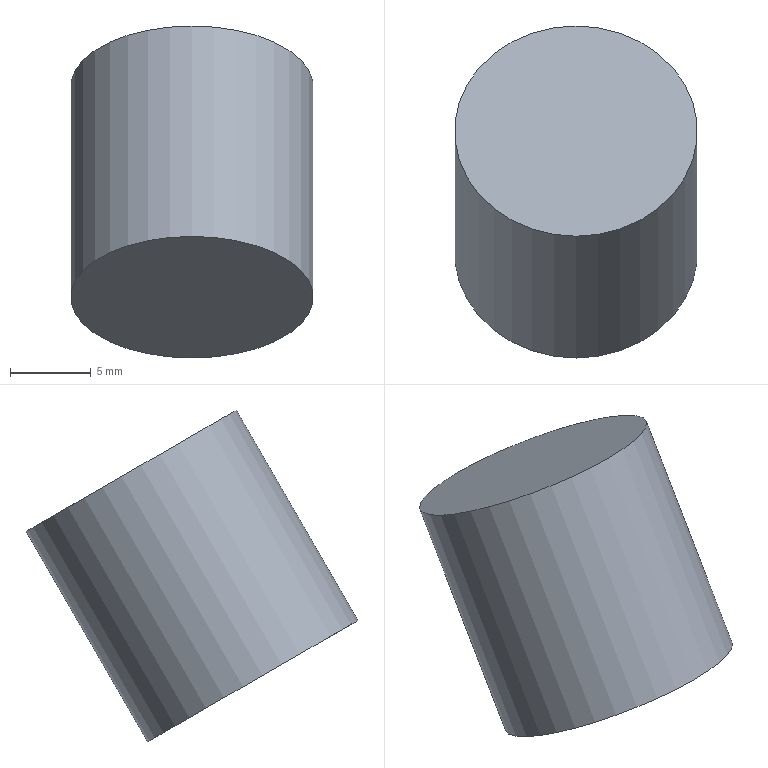Part | NX | features solid 2 | 1 solid | 3 faces | box 15 x 20.49 x 20.49 mm | volume 2651 mm3 | plane 2 | cylinder 1 | commonest cylinder face diameters 15 x1
STEP:
#1=CARTESIAN_POINT('',(335.,519.578,-155.064));
#2=VERTEX_POINT('',#1);
#3=CARTESIAN_POINT('',(335.,513.083,-151.314));
#4=DIRECTION('',(0.,0.5,0.866));
#5=DIRECTION('',(0.,0.866,-0.5));
#6=AXIS2_PLACEMENT_3D('',#3,#4,#5);
#7=CIRCLE('',#6,7.5);
#8=EDGE_CURVE('',#2,#2,#7,.T.);
#9=ORIENTED_EDGE('',*,*,#8,.F.);
#10=EDGE_LOOP('',(#9));
#11=FACE_BOUND('',#10,.T.);
#12=CARTESIAN_POINT('',(335.,512.078,-168.054));
#13=VERTEX_POINT('',#12);
#14=CARTESIAN_POINT('',(335.,505.583,-164.304));
#15=DIRECTION('',(0.,0.5,0.866));
#16=DIRECTION('',(0.,0.866,-0.5));
#17=AXIS2_PLACEMENT_3D('',#14,#15,#16);
#18=CIRCLE('',#17,7.5);
#19=EDGE_CURVE('',#13,#13,#18,.T.);
#20=ORIENTED_EDGE('',*,*,#19,.T.);
#21=EDGE_LOOP('',(#20));
#22=FACE_BOUND('',#21,.T.);
#23=CARTESIAN_POINT('',(335.,513.083,-151.314));
#24=DIRECTION('',(0.,-0.5,-0.866));
#25=DIRECTION('',(0.,-0.866,0.5));
#26=AXIS2_PLACEMENT_3D('',#23,#24,#25);
#27=CYLINDRICAL_SURFACE('',#26,7.5);
#28=ADVANCED_FACE('',(#11,#22),#27,.T.);
#29=ORIENTED_EDGE('',*,*,#8,.T.);
#30=EDGE_LOOP('',(#29));
#31=FACE_BOUND('',#30,.T.);
#32=CARTESIAN_POINT('',(335.,513.083,-151.314));
#33=DIRECTION('',(0.,0.5,0.866));
#34=DIRECTION('',(0.,0.866,-0.5));
#35=AXIS2_PLACEMENT_3D('',#32,#33,#34);
#36=PLANE('',#35);
#37=ADVANCED_FACE('',(#31),#36,.T.);
#38=ORIENTED_EDGE('',*,*,#19,.F.);
#39=EDGE_LOOP('',(#38));
#40=FACE_BOUND('',#39,.T.);
#41=CARTESIAN_POINT('',(335.,505.583,-164.304));
#42=DIRECTION('',(0.,0.5,0.866));
#43=DIRECTION('',(0.,0.866,-0.5));
#44=AXIS2_PLACEMENT_3D('',#41,#42,#43);
#45=PLANE('',#44);
#46=ADVANCED_FACE('',(#40),#45,.F.);
#47=CLOSED_SHELL('',(#28,#37,#46));
#48=MANIFOLD_SOLID_BREP('',#47);
#49=(LENGTH_UNIT()NAMED_UNIT(*)SI_UNIT(.MILLI.,.METRE.));
#50=UNCERTAINTY_MEASURE_WITH_UNIT(LENGTH_MEASURE(0.00001),#49,'','');
#51=(NAMED_UNIT(*)PLANE_ANGLE_UNIT()SI_UNIT($,.RADIAN.));
#52=(NAMED_UNIT(*)SI_UNIT($,.STERADIAN.)SOLID_ANGLE_UNIT());
#53=(GEOMETRIC_REPRESENTATION_CONTEXT(3)GLOBAL_UNCERTAINTY_ASSIGNED_CONTEXT((#50))GLOBAL_UNIT_ASSIGNED_CONTEXT((#49,#51,#52))REPRESENTATION_CONTEXT('',''));
#54=ADVANCED_BREP_SHAPE_REPRESENTATION('',(#48),#53);